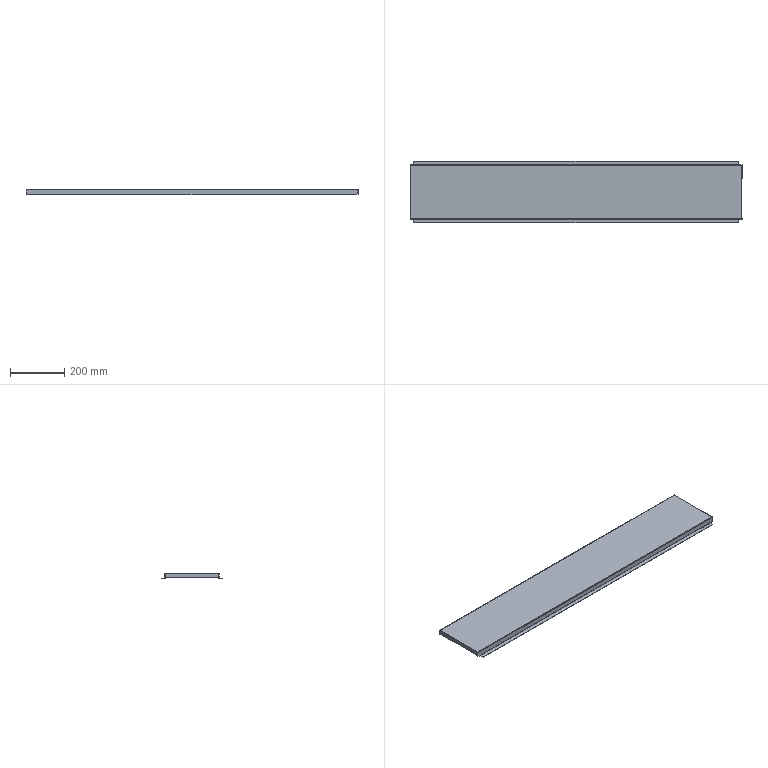Part | SolidWorks | features EdgeFlange 3, FlatPattern 1, ICE 1, SMBaseFlange 1, SheetMetal 1 | 1 solid | 66 faces | box 1220 x 227.6 x 21.2 mm | volume 394431 mm3 | plane 54 | cylinder 12 | commonest cylinder face diameters 0.9 x6 3.3 x6